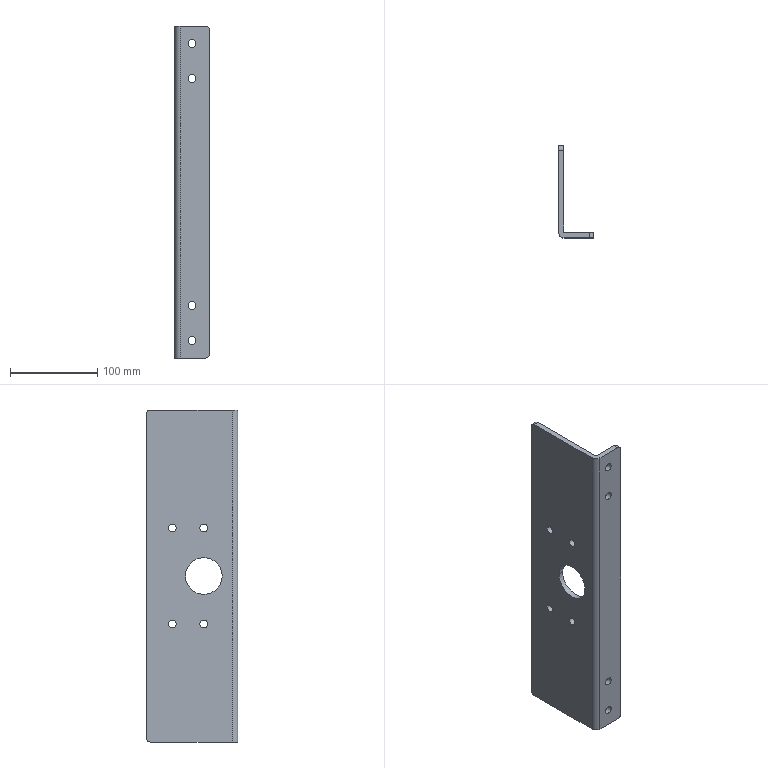Part | STEP file | 1 solid | 32 faces | box 40 x 105 x 380 mm | volume 302196 mm3 | cylinder 24 | plane 8 | commonest cylinder face diameters 9 x16 10 x4 42 x2 0.6 x1 12.6 x1